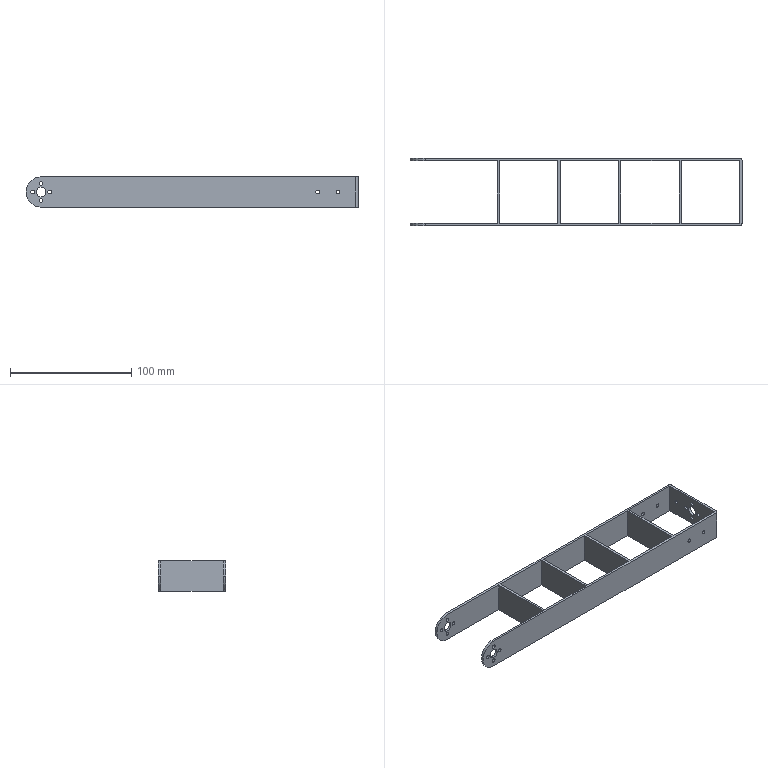Part | SolidWorks | features ICE 5, Fillet 3, Extrusion 1 | 1 solid | 72 faces | box 274.25 x 56 x 25 mm | volume 39558 mm3 | cylinder 48 | plane 24 | commonest cylinder face diameters 3 x36 8 x6 25 x4 4 x2